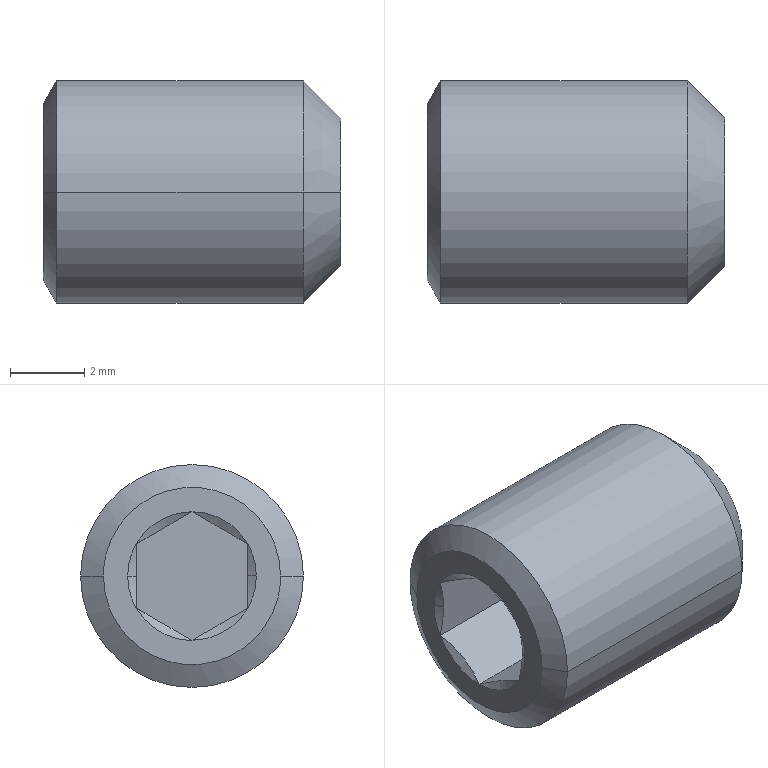Part | STEP file | _Headless pin DIN 913 - M6x8 | 1 solid | 23 faces | box 8 x 6 x 6 mm | volume 188.543 mm3 | cone 12 | plane 9 | cylinder 2 | commonest cylinder face diameters 6 x2
STEP:
#1=CARTESIAN_POINT('',(0.,-1.5,0.866));
#2=VERTEX_POINT('',#1);
#3=CARTESIAN_POINT('',(0.,0.,1.732));
#4=VERTEX_POINT('',#3);
#5=CARTESIAN_POINT('',(0.,-1.5,0.866));
#6=CARTESIAN_POINT('',(0.1211,-1.137,1.075));
#7=CARTESIAN_POINT('',(0.1533,-0.8845,1.221));
#8=CARTESIAN_POINT('',(0.1534,-0.6169,1.377));
#9=CARTESIAN_POINT('',(0.1211,-0.3629,1.522));
#10=CARTESIAN_POINT('',(0.,0.,1.732));
#11=B_SPLINE_CURVE_WITH_KNOTS('',5,(#5,#6,#7,#8,#9,#10),.UNSPECIFIED.,.F.,.U.,(6,6),(0.,104.781),.UNSPECIFIED.);
#12=EDGE_CURVE('',#2,#4,#11,.T.);
#13=ORIENTED_EDGE('',*,*,#12,.F.);
#14=CARTESIAN_POINT('',(0.,0.,0.));
#15=DIRECTION('',(-1.,0.,0.));
#16=AXIS2_PLACEMENT_3D('',#14,#15,$);
#17=CIRCLE('',#16,1.732);
#18=EDGE_CURVE('',#2,#4,#17,.T.);
#19=ORIENTED_EDGE('',*,*,#18,.T.);
#20=EDGE_LOOP('',(#13,#19));
#21=FACE_OUTER_BOUND('',#20,.T.);
#22=CARTESIAN_POINT('',(0.,0.,0.));
#23=DIRECTION('',(-1.,0.,0.));
#24=DIRECTION('',(0.,-1.,0.));
#25=AXIS2_PLACEMENT_3D('',#22,#23,#24);
#26=CONICAL_SURFACE('',#25,1.732,1.047);
#27=ADVANCED_FACE('',(#21),#26,.F.);
#28=ORIENTED_EDGE('',*,*,#12,.T.);
#29=CARTESIAN_POINT('',(3.5,-0.000000001,1.732));
#30=VERTEX_POINT('',#29);
#31=CARTESIAN_POINT('',(1.75,0.,1.732));
#32=DIRECTION('',(-1.,0.,0.));
#33=VECTOR('',#32,1.);
#34=LINE('',#31,#33);
#35=EDGE_CURVE('',#30,#4,#34,.T.);
#36=ORIENTED_EDGE('',*,*,#35,.F.);
#37=CARTESIAN_POINT('',(3.5,-1.5,0.866));
#38=VERTEX_POINT('',#37);
#39=CARTESIAN_POINT('',(3.5,-0.75,1.299));
#40=DIRECTION('',(0.,-0.866,-0.5));
#41=VECTOR('',#40,1.);
#42=LINE('',#39,#41);
#43=EDGE_CURVE('',#30,#38,#42,.T.);
#44=ORIENTED_EDGE('',*,*,#43,.T.);
#45=CARTESIAN_POINT('',(1.75,-1.5,0.866));
#46=DIRECTION('',(-1.,0.,0.));
#47=VECTOR('',#46,1.);
#48=LINE('',#45,#47);
#49=EDGE_CURVE('',#38,#2,#48,.T.);
#50=ORIENTED_EDGE('',*,*,#49,.T.);
#51=EDGE_LOOP('',(#28,#36,#44,#50));
#52=FACE_OUTER_BOUND('',#51,.T.);
#53=CARTESIAN_POINT('',(3.5,0.,1.732));
#54=DIRECTION('',(0.,0.5,-0.866));
#55=DIRECTION('',(0.,0.866,0.5));
#56=AXIS2_PLACEMENT_3D('',#53,#54,#55);
#57=PLANE('',#56);
#58=ADVANCED_FACE('',(#52),#57,.T.);
#59=CARTESIAN_POINT('',(0.,2.386,0.));
#60=VERTEX_POINT('',#59);
#61=CARTESIAN_POINT('',(0.,-2.386,0.));
#62=VERTEX_POINT('',#61);
#63=CARTESIAN_POINT('',(0.,2.387,0.));
#64=CARTESIAN_POINT('',(0.,2.387,-0.227));
#65=CARTESIAN_POINT('',(0.,2.36,-0.4541));
#66=CARTESIAN_POINT('',(0.,2.305,-0.6768));
#67=CARTESIAN_POINT('',(0.,2.146,-1.105));
#68=CARTESIAN_POINT('',(0.,1.89,-1.484));
#69=CARTESIAN_POINT('',(0.,1.74,-1.657));
#70=CARTESIAN_POINT('',(0.,1.401,-1.965));
#71=CARTESIAN_POINT('',(0.,1.,-2.185));
#72=CARTESIAN_POINT('',(0.,0.7874,-2.27));
#73=CARTESIAN_POINT('',(0.,0.3458,-2.389));
#74=CARTESIAN_POINT('',(0.,-0.1114,-2.4));
#75=CARTESIAN_POINT('',(0.,-0.3396,-2.379));
#76=CARTESIAN_POINT('',(0.,-0.7865,-2.282));
#77=CARTESIAN_POINT('',(0.,-1.198,-2.083));
#78=CARTESIAN_POINT('',(0.,-1.391,-1.959));
#79=CARTESIAN_POINT('',(0.,-1.744,-1.668));
#80=CARTESIAN_POINT('',(0.,-2.019,-1.303));
#81=CARTESIAN_POINT('',(0.,-2.134,-1.105));
#82=CARTESIAN_POINT('',(0.,-2.279,-0.7675));
#83=CARTESIAN_POINT('',(0.,-2.357,-0.4107));
#84=CARTESIAN_POINT('',(0.,-2.377,-0.2745));
#85=CARTESIAN_POINT('',(0.,-2.386,-0.1372));
#86=CARTESIAN_POINT('',(0.,-2.386,0.));
#87=B_SPLINE_CURVE_WITH_KNOTS('',5,(#63,#64,#65,#66,#67,#68,#69,#70,#71,#72,#73,#74,#75,#76,#77,#78,#79,#80,#81,#82,#83,#84,#85,#86),.UNSPECIFIED.,.F.,.U.,(6,3,3,3,3,3,3,6),(0.,1.605,3.211,4.816,6.422,8.027,9.633,10.603),.UNSPECIFIED.);
#88=EDGE_CURVE('',#60,#62,#87,.T.);
#89=ORIENTED_EDGE('',*,*,#88,.T.);
#90=CARTESIAN_POINT('',(0.,-2.386,0.));
#91=CARTESIAN_POINT('',(0.,-2.386,0.227));
#92=CARTESIAN_POINT('',(0.,-2.36,0.4541));
#93=CARTESIAN_POINT('',(0.,-2.305,0.6768));
#94=CARTESIAN_POINT('',(0.,-2.146,1.105));
#95=CARTESIAN_POINT('',(0.,-1.89,1.484));
#96=CARTESIAN_POINT('',(0.,-1.74,1.657));
#97=CARTESIAN_POINT('',(0.,-1.401,1.965));
#98=CARTESIAN_POINT('',(0.,-1.,2.185));
#99=CARTESIAN_POINT('',(0.,-0.7874,2.27));
#100=CARTESIAN_POINT('',(0.,-0.3458,2.389));
#101=CARTESIAN_POINT('',(0.,0.1114,2.4));
#102=CARTESIAN_POINT('',(0.,0.3396,2.379));
#103=CARTESIAN_POINT('',(0.,0.7865,2.282));
#104=CARTESIAN_POINT('',(0.,1.198,2.083));
#105=CARTESIAN_POINT('',(0.,1.391,1.959));
#106=CARTESIAN_POINT('',(0.,1.744,1.668));
#107=CARTESIAN_POINT('',(0.,2.019,1.303));
#108=CARTESIAN_POINT('',(0.,2.134,1.105));
#109=CARTESIAN_POINT('',(0.,2.279,0.7675));
#110=CARTESIAN_POINT('',(0.,2.357,0.4107));
#111=CARTESIAN_POINT('',(0.,2.377,0.2745));
#112=CARTESIAN_POINT('',(0.,2.387,0.1372));
#113=CARTESIAN_POINT('',(0.,2.387,0.));
#114=B_SPLINE_CURVE_WITH_KNOTS('',5,(#90,#91,#92,#93,#94,#95,#96,#97,#98,#99,#100,#101,#102,#103,#104,#105,#106,#107,#108,#109,#110,#111,#112,#113),.UNSPECIFIED.,.F.,.U.,(6,3,3,3,3,3,3,6),(0.,1.605,3.211,4.816,6.422,8.027,9.633,10.603),.UNSPECIFIED.);
#115=EDGE_CURVE('',#62,#60,#114,.T.);
#116=ORIENTED_EDGE('',*,*,#115,.T.);
#117=EDGE_LOOP('',(#89,#116));
#118=FACE_OUTER_BOUND('',#117,.T.);
#119=CARTESIAN_POINT('',(0.,-1.732,0.));
#120=VERTEX_POINT('',#119);
#121=CARTESIAN_POINT('',(0.,-1.732,0.));
#122=CARTESIAN_POINT('',(0.,-1.732,0.01204));
#123=CARTESIAN_POINT('',(0.,-1.732,0.02409));
#124=CARTESIAN_POINT('',(0.,-1.732,0.03613));
#125=CARTESIAN_POINT('',(0.,-1.727,0.2175));
#126=CARTESIAN_POINT('',(0.,-1.699,0.3979));
#127=CARTESIAN_POINT('',(0.,-1.651,0.5624));
#128=CARTESIAN_POINT('',(0.,-1.585,0.7194));
#129=CARTESIAN_POINT('',(0.,-1.5,0.866));
#130=B_SPLINE_CURVE_WITH_KNOTS('',5,(#121,#122,#123,#124,#125,#126,#127,#128,#129),.UNSPECIFIED.,.F.,.U.,(6,3,6),(1.283,1.368,2.565),.UNSPECIFIED.);
#131=EDGE_CURVE('',#120,#2,#130,.T.);
#132=ORIENTED_EDGE('',*,*,#131,.F.);
#133=CARTESIAN_POINT('',(0.,-1.5,-0.866));
#134=VERTEX_POINT('',#133);
#135=CARTESIAN_POINT('',(0.,-1.5,-0.866));
#136=CARTESIAN_POINT('',(0.,-1.591,-0.7089));
#137=CARTESIAN_POINT('',(0.,-1.661,-0.54));
#138=CARTESIAN_POINT('',(0.,-1.708,-0.3628));
#139=CARTESIAN_POINT('',(0.,-1.732,-0.1814));
#140=CARTESIAN_POINT('',(0.,-1.732,0.));
#141=B_SPLINE_CURVE_WITH_KNOTS('',5,(#135,#136,#137,#138,#139,#140),.UNSPECIFIED.,.F.,.U.,(6,6),(0.,1.283),.UNSPECIFIED.);
#142=EDGE_CURVE('',#134,#120,#141,.T.);
#143=ORIENTED_EDGE('',*,*,#142,.F.);
#144=CARTESIAN_POINT('',(0.,0.,-1.732));
#145=VERTEX_POINT('',#144);
#146=CARTESIAN_POINT('',(0.,-0.000000001,-1.732));
#147=CARTESIAN_POINT('',(0.,-0.1934,-1.732));
#148=CARTESIAN_POINT('',(0.,-0.3868,-1.705));
#149=CARTESIAN_POINT('',(0.,-0.5752,-1.651));
#150=CARTESIAN_POINT('',(0.,-0.9097,-1.502));
#151=CARTESIAN_POINT('',(0.,-1.194,-1.272));
#152=CARTESIAN_POINT('',(0.,-1.313,-1.149));
#153=CARTESIAN_POINT('',(0.,-1.415,-1.013));
#154=CARTESIAN_POINT('',(0.,-1.5,-0.866));
#155=B_SPLINE_CURVE_WITH_KNOTS('',5,(#146,#147,#148,#149,#150,#151,#152,#153,#154),.UNSPECIFIED.,.F.,.U.,(6,3,6),(0.,1.368,2.565),.UNSPECIFIED.);
#156=EDGE_CURVE('',#145,#134,#155,.T.);
#157=ORIENTED_EDGE('',*,*,#156,.F.);
#158=CARTESIAN_POINT('',(0.,1.5,-0.866));
#159=VERTEX_POINT('',#158);
#160=CARTESIAN_POINT('',(0.,1.5,-0.866));
#161=CARTESIAN_POINT('',(0.,1.403,-1.034));
#162=CARTESIAN_POINT('',(0.,1.283,-1.188));
#163=CARTESIAN_POINT('',(0.,1.142,-1.324));
#164=CARTESIAN_POINT('',(0.,0.8457,-1.539));
#165=CARTESIAN_POINT('',(0.,0.5046,-1.67));
#166=CARTESIAN_POINT('',(0.,0.3387,-1.711));
#167=CARTESIAN_POINT('',(0.,0.1693,-1.732));
#168=CARTESIAN_POINT('',(0.,-0.000000001,-1.732));
#169=B_SPLINE_CURVE_WITH_KNOTS('',5,(#160,#161,#162,#163,#164,#165,#166,#167,#168),.UNSPECIFIED.,.F.,.U.,(6,3,6),(0.,1.368,2.565),.UNSPECIFIED.);
#170=EDGE_CURVE('',#159,#145,#169,.T.);
#171=ORIENTED_EDGE('',*,*,#170,.F.);
#172=CARTESIAN_POINT('',(0.,1.732,0.));
#173=VERTEX_POINT('',#172);
#174=CARTESIAN_POINT('',(0.,1.732,0.));
#175=CARTESIAN_POINT('',(0.,1.732,-0.01204));
#176=CARTESIAN_POINT('',(0.,1.732,-0.02409));
#177=CARTESIAN_POINT('',(0.,1.732,-0.03613));
#178=CARTESIAN_POINT('',(0.,1.727,-0.2175));
#179=CARTESIAN_POINT('',(0.,1.699,-0.3979));
#180=CARTESIAN_POINT('',(0.,1.651,-0.5624));
#181=CARTESIAN_POINT('',(0.,1.585,-0.7194));
#182=CARTESIAN_POINT('',(0.,1.5,-0.866));
#183=B_SPLINE_CURVE_WITH_KNOTS('',5,(#174,#175,#176,#177,#178,#179,#180,#181,#182),.UNSPECIFIED.,.F.,.U.,(6,3,6),(1.283,1.368,2.565),.UNSPECIFIED.);
#184=EDGE_CURVE('',#173,#159,#183,.T.);
#185=ORIENTED_EDGE('',*,*,#184,.F.);
#186=CARTESIAN_POINT('',(0.,1.5,0.866));
#187=VERTEX_POINT('',#186);
#188=CARTESIAN_POINT('',(0.,1.5,0.866));
#189=CARTESIAN_POINT('',(0.,1.591,0.7089));
#190=CARTESIAN_POINT('',(0.,1.661,0.54));
#191=CARTESIAN_POINT('',(0.,1.708,0.3628));
#192=CARTESIAN_POINT('',(0.,1.732,0.1814));
#193=CARTESIAN_POINT('',(0.,1.732,0.));
#194=B_SPLINE_CURVE_WITH_KNOTS('',5,(#188,#189,#190,#191,#192,#193),.UNSPECIFIED.,.F.,.U.,(6,6),(0.,1.283),.UNSPECIFIED.);
#195=EDGE_CURVE('',#187,#173,#194,.T.);
#196=ORIENTED_EDGE('',*,*,#195,.F.);
#197=CARTESIAN_POINT('',(0.,-0.000000001,1.732));
#198=CARTESIAN_POINT('',(0.,0.1934,1.732));
#199=CARTESIAN_POINT('',(0.,0.3868,1.705));
#200=CARTESIAN_POINT('',(0.,0.5752,1.651));
#201=CARTESIAN_POINT('',(0.,0.9097,1.502));
#202=CARTESIAN_POINT('',(0.,1.194,1.272));
#203=CARTESIAN_POINT('',(0.,1.313,1.149));
#204=CARTESIAN_POINT('',(0.,1.415,1.013));
#205=CARTESIAN_POINT('',(0.,1.5,0.866));
#206=B_SPLINE_CURVE_WITH_KNOTS('',5,(#197,#198,#199,#200,#201,#202,#203,#204,#205),.UNSPECIFIED.,.F.,.U.,(6,3,6),(0.,1.368,2.565),.UNSPECIFIED.);
#207=EDGE_CURVE('',#4,#187,#206,.T.);
#208=ORIENTED_EDGE('',*,*,#207,.F.);
#209=ORIENTED_EDGE('',*,*,#18,.F.);
#210=EDGE_LOOP('',(#132,#143,#157,#171,#185,#196,#208,#209));
#211=FACE_BOUND('',#210,.T.);
#212=CARTESIAN_POINT('',(0.,-2.386,0.));
#213=DIRECTION('',(1.,0.,0.));
#214=DIRECTION('',(0.,1.,0.));
#215=AXIS2_PLACEMENT_3D('',#212,#213,#214);
#216=PLANE('',#215);
#217=ADVANCED_FACE('',(#118,#211),#216,.F.);
#218=CARTESIAN_POINT('',(0.,-0.000000001,1.732));
#219=CARTESIAN_POINT('',(0.05807,0.1735,1.632));
#220=CARTESIAN_POINT('',(0.1037,0.3502,1.53));
#221=CARTESIAN_POINT('',(0.1362,0.5392,1.421));
#222=CARTESIAN_POINT('',(0.1461,0.8424,1.246));
#223=CARTESIAN_POINT('',(0.0996,1.143,1.072));
#224=CARTESIAN_POINT('',(0.07278,1.264,1.002));
#225=CARTESIAN_POINT('',(0.03928,1.383,0.9336));
#226=CARTESIAN_POINT('',(0.,1.5,0.866));
#227=B_SPLINE_CURVE_WITH_KNOTS('',5,(#218,#219,#220,#221,#222,#223,#224,#225,#226),.UNSPECIFIED.,.F.,.U.,(6,3,6),(0.,1.478,2.475),.UNSPECIFIED.);
#228=EDGE_CURVE('',#4,#187,#227,.T.);
#229=ORIENTED_EDGE('',*,*,#228,.T.);
#230=CARTESIAN_POINT('',(3.5,1.5,0.866));
#231=VERTEX_POINT('',#230);
#232=CARTESIAN_POINT('',(1.75,1.5,0.866));
#233=DIRECTION('',(-1.,0.,0.));
#234=VECTOR('',#233,1.);
#235=LINE('',#232,#234);
#236=EDGE_CURVE('',#231,#187,#235,.T.);
#237=ORIENTED_EDGE('',*,*,#236,.F.);
#238=CARTESIAN_POINT('',(3.5,0.75,1.299));
#239=DIRECTION('',(0.,-0.866,0.5));
#240=VECTOR('',#239,1.);
#241=LINE('',#238,#240);
#242=EDGE_CURVE('',#231,#30,#241,.T.);
#243=ORIENTED_EDGE('',*,*,#242,.T.);
#244=ORIENTED_EDGE('',*,*,#35,.T.);
#245=EDGE_LOOP('',(#229,#237,#243,#244));
#246=FACE_OUTER_BOUND('',#245,.T.);
#247=CARTESIAN_POINT('',(3.5,1.5,0.866));
#248=DIRECTION('',(0.,-0.5,-0.866));
#249=DIRECTION('',(0.,0.866,-0.5));
#250=AXIS2_PLACEMENT_3D('',#247,#248,#249);
#251=PLANE('',#250);
#252=ADVANCED_FACE('',(#246),#251,.T.);
#253=ORIENTED_EDGE('',*,*,#242,.F.);
#254=CARTESIAN_POINT('',(3.5,1.5,-0.866));
#255=VERTEX_POINT('',#254);
#256=CARTESIAN_POINT('',(3.5,1.5,0.));
#257=DIRECTION('',(0.,0.,1.));
#258=VECTOR('',#257,1.);
#259=LINE('',#256,#258);
#260=EDGE_CURVE('',#255,#231,#259,.T.);
#261=ORIENTED_EDGE('',*,*,#260,.F.);
#262=CARTESIAN_POINT('',(3.5,0.000000001,-1.732));
#263=VERTEX_POINT('',#262);
#264=CARTESIAN_POINT('',(3.5,0.75,-1.299));
#265=DIRECTION('',(0.,0.866,0.5));
#266=VECTOR('',#265,1.);
#267=LINE('',#264,#266);
#268=EDGE_CURVE('',#263,#255,#267,.T.);
#269=ORIENTED_EDGE('',*,*,#268,.F.);
#270=CARTESIAN_POINT('',(3.5,-1.5,-0.866));
#271=VERTEX_POINT('',#270);
#272=CARTESIAN_POINT('',(3.5,-0.75,-1.299));
#273=DIRECTION('',(0.,0.866,-0.5));
#274=VECTOR('',#273,1.);
#275=LINE('',#272,#274);
#276=EDGE_CURVE('',#271,#263,#275,.T.);
#277=ORIENTED_EDGE('',*,*,#276,.F.);
#278=CARTESIAN_POINT('',(3.5,-1.5,0.));
#279=DIRECTION('',(0.,0.,-1.));
#280=VECTOR('',#279,1.);
#281=LINE('',#278,#280);
#282=EDGE_CURVE('',#38,#271,#281,.T.);
#283=ORIENTED_EDGE('',*,*,#282,.F.);
#284=ORIENTED_EDGE('',*,*,#43,.F.);
#285=EDGE_LOOP('',(#253,#261,#269,#277,#283,#284));
#286=FACE_OUTER_BOUND('',#285,.T.);
#287=CARTESIAN_POINT('',(3.5,0.,0.));
#288=DIRECTION('',(1.,0.,0.));
#289=DIRECTION('',(0.,0.,-1.));
#290=AXIS2_PLACEMENT_3D('',#287,#288,#289);
#291=PLANE('',#290);
#292=ADVANCED_FACE('',(#286),#291,.F.);
#293=CARTESIAN_POINT('',(0.134,-1.5,0.000000006));
#294=VERTEX_POINT('',#293);
#295=CARTESIAN_POINT('',(0.,-1.5,-0.866));
#296=CARTESIAN_POINT('',(0.03911,-1.5,-0.7307));
#297=CARTESIAN_POINT('',(0.07296,-1.5,-0.5931));
#298=CARTESIAN_POINT('',(0.1,-1.5,-0.455));
#299=CARTESIAN_POINT('',(0.1233,-1.5,-0.2807));
#300=CARTESIAN_POINT('',(0.1322,-1.5,-0.1053));
#301=CARTESIAN_POINT('',(0.1334,-1.5,-0.07031));
#302=CARTESIAN_POINT('',(0.134,-1.5,-0.0352));
#303=CARTESIAN_POINT('',(0.134,-1.5,-0.00000002));
#304=B_SPLINE_CURVE_WITH_KNOTS('',5,(#295,#296,#297,#298,#299,#300,#301,#302,#303),.UNSPECIFIED.,.F.,.U.,(6,3,6),(0.,0.997,1.245),.UNSPECIFIED.);
#305=EDGE_CURVE('',#134,#294,#304,.T.);
#306=ORIENTED_EDGE('',*,*,#305,.T.);
#307=CARTESIAN_POINT('',(0.134,-1.5,-0.00000002));
#308=CARTESIAN_POINT('',(0.1339,-1.5,0.1056));
#309=CARTESIAN_POINT('',(0.1284,-1.5,0.2121));
#310=CARTESIAN_POINT('',(0.1175,-1.5,0.3189));
#311=CARTESIAN_POINT('',(0.09166,-1.5,0.4924));
#312=CARTESIAN_POINT('',(0.05418,-1.5,0.6632));
#313=CARTESIAN_POINT('',(0.03749,-1.5,0.7312));
#314=CARTESIAN_POINT('',(0.01936,-1.5,0.7988));
#315=CARTESIAN_POINT('',(0.,-1.5,0.866));
#316=B_SPLINE_CURVE_WITH_KNOTS('',5,(#307,#308,#309,#310,#311,#312,#313,#314,#315),.UNSPECIFIED.,.F.,.U.,(6,3,6),(1.245,1.987,2.484),.UNSPECIFIED.);
#317=EDGE_CURVE('',#294,#2,#316,.T.);
#318=ORIENTED_EDGE('',*,*,#317,.T.);
#319=ORIENTED_EDGE('',*,*,#49,.F.);
#320=ORIENTED_EDGE('',*,*,#282,.T.);
#321=CARTESIAN_POINT('',(1.75,-1.5,-0.866));
#322=DIRECTION('',(-1.,0.,0.));
#323=VECTOR('',#322,1.);
#324=LINE('',#321,#323);
#325=EDGE_CURVE('',#271,#134,#324,.T.);
#326=ORIENTED_EDGE('',*,*,#325,.T.);
#327=EDGE_LOOP('',(#306,#318,#319,#320,#326));
#328=FACE_OUTER_BOUND('',#327,.T.);
#329=CARTESIAN_POINT('',(3.5,-1.5,0.866));
#330=DIRECTION('',(0.,1.,0.));
#331=DIRECTION('',(0.,0.,1.));
#332=AXIS2_PLACEMENT_3D('',#329,#330,#331);
#333=PLANE('',#332);
#334=ADVANCED_FACE('',(#328),#333,.T.);
#335=CARTESIAN_POINT('',(0.3542,-3.,0.));
#336=VERTEX_POINT('',#335);
#337=CARTESIAN_POINT('',(249999.488,-433014.202,0.));
#338=DIRECTION('',(0.5,-0.866,0.));
#339=VECTOR('',#338,1.);
#340=LINE('',#337,#339);
#341=EDGE_CURVE('',#62,#336,#340,.T.);
#342=ORIENTED_EDGE('',*,*,#341,.F.);
#343=ORIENTED_EDGE('',*,*,#88,.F.);
#344=CARTESIAN_POINT('',(0.3542,3.,0.));
#345=VERTEX_POINT('',#344);
#346=CARTESIAN_POINT('',(249999.488,433014.202,0.));
#347=DIRECTION('',(0.5,0.866,0.));
#348=VECTOR('',#347,1.);
#349=LINE('',#346,#348);
#350=EDGE_CURVE('',#345,#60,#349,.F.);
#351=ORIENTED_EDGE('',*,*,#350,.F.);
#352=CARTESIAN_POINT('',(0.3542,0.,0.));
#353=DIRECTION('',(1.,0.,0.));
#354=AXIS2_PLACEMENT_3D('',#352,#353,$);
#355=CIRCLE('',#354,3.);
#356=EDGE_CURVE('',#345,#336,#355,.F.);
#357=ORIENTED_EDGE('',*,*,#356,.T.);
#358=EDGE_LOOP('',(#342,#343,#351,#357));
#359=FACE_OUTER_BOUND('',#358,.T.);
#360=CARTESIAN_POINT('',(0.3542,0.,0.));
#361=DIRECTION('',(1.,0.,0.));
#362=DIRECTION('',(0.,-1.,0.));
#363=AXIS2_PLACEMENT_3D('',#360,#361,#362);
#364=CONICAL_SURFACE('',#363,3.,1.047);
#365=ADVANCED_FACE('',(#359),#364,.T.);
#366=ORIENTED_EDGE('',*,*,#350,.T.);
#367=ORIENTED_EDGE('',*,*,#115,.F.);
#368=ORIENTED_EDGE('',*,*,#341,.T.);
#369=CARTESIAN_POINT('',(0.3542,0.,0.));
#370=DIRECTION('',(1.,0.,0.));
#371=AXIS2_PLACEMENT_3D('',#369,#370,$);
#372=CIRCLE('',#371,3.);
#373=EDGE_CURVE('',#336,#345,#372,.F.);
#374=ORIENTED_EDGE('',*,*,#373,.T.);
#375=EDGE_LOOP('',(#366,#367,#368,#374));
#376=FACE_OUTER_BOUND('',#375,.T.);
#377=CARTESIAN_POINT('',(0.3542,0.,0.));
#378=DIRECTION('',(1.,0.,0.));
#379=DIRECTION('',(0.,1.,0.));
#380=AXIS2_PLACEMENT_3D('',#377,#378,#379);
#381=CONICAL_SURFACE('',#380,3.,1.047);
#382=ADVANCED_FACE('',(#376),#381,.T.);
#383=ORIENTED_EDGE('',*,*,#131,.T.);
#384=ORIENTED_EDGE('',*,*,#317,.F.);
#385=CARTESIAN_POINT('',(-249999.5,-433013.568,0.));
#386=DIRECTION('',(-0.5,-0.866,0.));
#387=VECTOR('',#386,1.);
#388=LINE('',#385,#387);
#389=EDGE_CURVE('',#120,#294,#388,.F.);
#390=ORIENTED_EDGE('',*,*,#389,.F.);
#391=EDGE_LOOP('',(#383,#384,#390));
#392=FACE_OUTER_BOUND('',#391,.T.);
#393=CARTESIAN_POINT('',(0.,0.,0.));
#394=DIRECTION('',(-1.,0.,0.));
#395=DIRECTION('',(0.,-1.,0.));
#396=AXIS2_PLACEMENT_3D('',#393,#394,#395);
#397=CONICAL_SURFACE('',#396,1.732,1.047);
#398=ADVANCED_FACE('',(#392),#397,.F.);
#399=ORIENTED_EDGE('',*,*,#305,.F.);
#400=ORIENTED_EDGE('',*,*,#142,.T.);
#401=ORIENTED_EDGE('',*,*,#389,.T.);
#402=EDGE_LOOP('',(#399,#400,#401));
#403=FACE_OUTER_BOUND('',#402,.T.);
#404=CARTESIAN_POINT('',(0.,0.,0.));
#405=DIRECTION('',(-1.,0.,0.));
#406=DIRECTION('',(0.,1.,0.));
#407=AXIS2_PLACEMENT_3D('',#404,#405,#406);
#408=CONICAL_SURFACE('',#407,1.732,1.047);
#409=ADVANCED_FACE('',(#403),#408,.F.);
#410=CARTESIAN_POINT('',(0.,0.,-1.732));
#411=CARTESIAN_POINT('',(0.1211,-0.3629,-1.522));
#412=CARTESIAN_POINT('',(0.1533,-0.6156,-1.377));
#413=CARTESIAN_POINT('',(0.1534,-0.8837,-1.223));
#414=CARTESIAN_POINT('',(0.1211,-1.137,-1.075));
#415=CARTESIAN_POINT('',(0.,-1.5,-0.866));
#416=B_SPLINE_CURVE_WITH_KNOTS('',5,(#410,#411,#412,#413,#414,#415),.UNSPECIFIED.,.F.,.U.,(6,6),(0.,104.781),.UNSPECIFIED.);
#417=EDGE_CURVE('',#145,#134,#416,.T.);
#418=ORIENTED_EDGE('',*,*,#417,.F.);
#419=ORIENTED_EDGE('',*,*,#156,.T.);
#420=EDGE_LOOP('',(#418,#419));
#421=FACE_OUTER_BOUND('',#420,.T.);
#422=CARTESIAN_POINT('',(0.,0.,0.));
#423=DIRECTION('',(-1.,0.,0.));
#424=DIRECTION('',(0.,1.,0.));
#425=AXIS2_PLACEMENT_3D('',#422,#423,#424);
#426=CONICAL_SURFACE('',#425,1.732,1.047);
#427=ADVANCED_FACE('',(#421),#426,.F.);
#428=CARTESIAN_POINT('',(0.,1.5,-0.866));
#429=CARTESIAN_POINT('',(0.1211,1.137,-1.075));
#430=CARTESIAN_POINT('',(0.1533,0.8845,-1.221));
#431=CARTESIAN_POINT('',(0.1534,0.6169,-1.377));
#432=CARTESIAN_POINT('',(0.1211,0.3629,-1.522));
#433=CARTESIAN_POINT('',(0.,0.,-1.732));
#434=B_SPLINE_CURVE_WITH_KNOTS('',5,(#428,#429,#430,#431,#432,#433),.UNSPECIFIED.,.F.,.U.,(6,6),(0.,104.781),.UNSPECIFIED.);
#435=EDGE_CURVE('',#159,#145,#434,.T.);
#436=ORIENTED_EDGE('',*,*,#435,.F.);
#437=ORIENTED_EDGE('',*,*,#170,.T.);
#438=EDGE_LOOP('',(#436,#437));
#439=FACE_OUTER_BOUND('',#438,.T.);
#440=CARTESIAN_POINT('',(0.,0.,0.));
#441=DIRECTION('',(-1.,0.,0.));
#442=DIRECTION('',(0.,1.,0.));
#443=AXIS2_PLACEMENT_3D('',#440,#441,#442);
#444=CONICAL_SURFACE('',#443,1.732,1.047);
#445=ADVANCED_FACE('',(#439),#444,.F.);
#446=ORIENTED_EDGE('',*,*,#184,.T.);
#447=CARTESIAN_POINT('',(0.134,1.5,0.));
#448=VERTEX_POINT('',#447);
#449=CARTESIAN_POINT('',(0.,1.5,-0.866));
#450=CARTESIAN_POINT('',(0.07581,1.5,-0.6035));
#451=CARTESIAN_POINT('',(0.1136,1.5,-0.3939));
#452=CARTESIAN_POINT('',(0.134,1.5,-0.1969));
#453=CARTESIAN_POINT('',(0.134,1.5,0.));
#454=B_SPLINE_CURVE_WITH_KNOTS('',4,(#449,#450,#451,#452,#453),.UNSPECIFIED.,.F.,.U.,(5,5),(0.,52.521),.UNSPECIFIED.);
#455=EDGE_CURVE('',#448,#159,#454,.F.);
#456=ORIENTED_EDGE('',*,*,#455,.F.);
#457=CARTESIAN_POINT('',(-249999.5,433013.568,0.));
#458=DIRECTION('',(-0.5,0.866,0.));
#459=VECTOR('',#458,1.);
#460=LINE('',#457,#459);
#461=EDGE_CURVE('',#448,#173,#460,.T.);
#462=ORIENTED_EDGE('',*,*,#461,.T.);
#463=EDGE_LOOP('',(#446,#456,#462));
#464=FACE_OUTER_BOUND('',#463,.T.);
#465=CARTESIAN_POINT('',(0.,0.,0.));
#466=DIRECTION('',(-1.,0.,0.));
#467=DIRECTION('',(0.,1.,0.));
#468=AXIS2_PLACEMENT_3D('',#465,#466,#467);
#469=CONICAL_SURFACE('',#468,1.732,1.047);
#470=ADVANCED_FACE('',(#464),#469,.F.);
#471=CARTESIAN_POINT('',(0.134,1.5,0.));
#472=CARTESIAN_POINT('',(0.1339,1.5,0.1962));
#473=CARTESIAN_POINT('',(0.1137,1.5,0.3943));
#474=CARTESIAN_POINT('',(0.07547,1.5,0.6045));
#475=CARTESIAN_POINT('',(0.,1.5,0.866));
#476=B_SPLINE_CURVE_WITH_KNOTS('',4,(#471,#472,#473,#474,#475),.UNSPECIFIED.,.F.,.U.,(5,5),(0.,52.333),.UNSPECIFIED.);
#477=EDGE_CURVE('',#187,#448,#476,.F.);
#478=ORIENTED_EDGE('',*,*,#477,.F.);
#479=ORIENTED_EDGE('',*,*,#195,.T.);
#480=ORIENTED_EDGE('',*,*,#461,.F.);
#481=EDGE_LOOP('',(#478,#479,#480));
#482=FACE_OUTER_BOUND('',#481,.T.);
#483=CARTESIAN_POINT('',(0.,0.,0.));
#484=DIRECTION('',(-1.,0.,0.));
#485=DIRECTION('',(0.,-1.,0.));
#486=AXIS2_PLACEMENT_3D('',#483,#484,#485);
#487=CONICAL_SURFACE('',#486,1.732,1.047);
#488=ADVANCED_FACE('',(#482),#487,.F.);
#489=ORIENTED_EDGE('',*,*,#228,.F.);
#490=ORIENTED_EDGE('',*,*,#207,.T.);
#491=EDGE_LOOP('',(#489,#490));
#492=FACE_OUTER_BOUND('',#491,.T.);
#493=CARTESIAN_POINT('',(0.,0.,0.));
#494=DIRECTION('',(-1.,0.,0.));
#495=DIRECTION('',(0.,-1.,0.));
#496=AXIS2_PLACEMENT_3D('',#493,#494,#495);
#497=CONICAL_SURFACE('',#496,1.732,1.047);
#498=ADVANCED_FACE('',(#492),#497,.F.);
#499=ORIENTED_EDGE('',*,*,#477,.T.);
#500=ORIENTED_EDGE('',*,*,#455,.T.);
#501=CARTESIAN_POINT('',(1.75,1.5,-0.866));
#502=DIRECTION('',(-1.,0.,0.));
#503=VECTOR('',#502,1.);
#504=LINE('',#501,#503);
#505=EDGE_CURVE('',#255,#159,#504,.T.);
#506=ORIENTED_EDGE('',*,*,#505,.F.);
#507=ORIENTED_EDGE('',*,*,#260,.T.);
#508=ORIENTED_EDGE('',*,*,#236,.T.);
#509=EDGE_LOOP('',(#499,#500,#506,#507,#508));
#510=FACE_OUTER_BOUND('',#509,.T.);
#511=CARTESIAN_POINT('',(3.5,1.5,-0.866));
#512=DIRECTION('',(0.,-1.,0.));
#513=DIRECTION('',(0.,0.,-1.));
#514=AXIS2_PLACEMENT_3D('',#511,#512,#513);
#515=PLANE('',#514);
#516=ADVANCED_FACE('',(#510),#515,.T.);
#517=ORIENTED_EDGE('',*,*,#435,.T.);
#518=CARTESIAN_POINT('',(1.75,0.,-1.732));
#519=DIRECTION('',(-1.,0.,0.));
#520=VECTOR('',#519,1.);
#521=LINE('',#518,#520);
#522=EDGE_CURVE('',#263,#145,#521,.T.);
#523=ORIENTED_EDGE('',*,*,#522,.F.);
#524=ORIENTED_EDGE('',*,*,#268,.T.);
#525=ORIENTED_EDGE('',*,*,#505,.T.);
#526=EDGE_LOOP('',(#517,#523,#524,#525));
#527=FACE_OUTER_BOUND('',#526,.T.);
#528=CARTESIAN_POINT('',(3.5,0.,-1.732));
#529=DIRECTION('',(0.,-0.5,0.866));
#530=DIRECTION('',(0.,-0.866,-0.5));
#531=AXIS2_PLACEMENT_3D('',#528,#529,#530);
#532=PLANE('',#531);
#533=ADVANCED_FACE('',(#527),#532,.T.);
#534=ORIENTED_EDGE('',*,*,#417,.T.);
#535=ORIENTED_EDGE('',*,*,#325,.F.);
#536=ORIENTED_EDGE('',*,*,#276,.T.);
#537=ORIENTED_EDGE('',*,*,#522,.T.);
#538=EDGE_LOOP('',(#534,#535,#536,#537));
#539=FACE_OUTER_BOUND('',#538,.T.);
#540=CARTESIAN_POINT('',(3.5,-1.5,-0.866));
#541=DIRECTION('',(0.,0.5,0.866));
#542=DIRECTION('',(0.,-0.866,0.5));
#543=AXIS2_PLACEMENT_3D('',#540,#541,#542);
#544=PLANE('',#543);
#545=ADVANCED_FACE('',(#539),#544,.T.);
#546=CARTESIAN_POINT('',(7.,3.,0.));
#547=VERTEX_POINT('',#546);
#548=CARTESIAN_POINT('',(1.,3.,0.));
#549=DIRECTION('',(1.,0.,0.));
#550=VECTOR('',#549,1.);
#551=LINE('',#548,#550);
#552=EDGE_CURVE('',#345,#547,#551,.T.);
#553=ORIENTED_EDGE('',*,*,#552,.T.);
#554=CARTESIAN_POINT('',(7.,-3.,0.));
#555=VERTEX_POINT('',#554);
#556=CARTESIAN_POINT('',(7.,0.,0.));
#557=DIRECTION('',(1.,0.,0.));
#558=AXIS2_PLACEMENT_3D('',#556,#557,$);
#559=CIRCLE('',#558,3.);
#560=EDGE_CURVE('',#547,#555,#559,.F.);
#561=ORIENTED_EDGE('',*,*,#560,.T.);
#562=CARTESIAN_POINT('',(1.,-3.,0.));
#563=DIRECTION('',(1.,0.,0.));
#564=VECTOR('',#563,1.);
#565=LINE('',#562,#564);
#566=EDGE_CURVE('',#555,#336,#565,.F.);
#567=ORIENTED_EDGE('',*,*,#566,.T.);
#568=ORIENTED_EDGE('',*,*,#356,.F.);
#569=EDGE_LOOP('',(#553,#561,#567,#568));
#570=FACE_OUTER_BOUND('',#569,.T.);
#571=CARTESIAN_POINT('',(1.,0.,0.));
#572=DIRECTION('',(1.,0.,0.));
#573=DIRECTION('',(0.,-1.,0.));
#574=AXIS2_PLACEMENT_3D('',#571,#572,#573);
#575=CYLINDRICAL_SURFACE('',#574,3.);
#576=ADVANCED_FACE('',(#570),#575,.T.);
#577=ORIENTED_EDGE('',*,*,#566,.F.);
#578=CARTESIAN_POINT('',(7.,0.,0.));
#579=DIRECTION('',(1.,0.,0.));
#580=AXIS2_PLACEMENT_3D('',#578,#579,$);
#581=CIRCLE('',#580,3.);
#582=EDGE_CURVE('',#555,#547,#581,.F.);
#583=ORIENTED_EDGE('',*,*,#582,.T.);
#584=ORIENTED_EDGE('',*,*,#552,.F.);
#585=ORIENTED_EDGE('',*,*,#373,.F.);
#586=EDGE_LOOP('',(#577,#583,#584,#585));
#587=FACE_OUTER_BOUND('',#586,.T.);
#588=CARTESIAN_POINT('',(1.,0.,0.));
#589=DIRECTION('',(1.,0.,0.));
#590=DIRECTION('',(0.,1.,0.));
#591=AXIS2_PLACEMENT_3D('',#588,#589,#590);
#592=CYLINDRICAL_SURFACE('',#591,3.);
#593=ADVANCED_FACE('',(#587),#592,.T.);
#594=CARTESIAN_POINT('',(8.,2.,0.));
#595=VERTEX_POINT('',#594);
#596=CARTESIAN_POINT('',(-353544.391,353554.391,0.));
#597=DIRECTION('',(-0.7071,0.7071,0.));
#598=VECTOR('',#597,1.);
#599=LINE('',#596,#598);
#600=EDGE_CURVE('',#595,#547,#599,.T.);
#601=ORIENTED_EDGE('',*,*,#600,.F.);
#602=CARTESIAN_POINT('',(8.,-2.,0.));
#603=VERTEX_POINT('',#602);
#604=CARTESIAN_POINT('',(8.,0.,0.));
#605=DIRECTION('',(-1.,0.,0.));
#606=AXIS2_PLACEMENT_3D('',#604,#605,$);
#607=CIRCLE('',#606,2.);
#608=EDGE_CURVE('',#595,#603,#607,.T.);
#609=ORIENTED_EDGE('',*,*,#608,.T.);
#610=CARTESIAN_POINT('',(-353544.391,-353554.391,0.));
#611=DIRECTION('',(-0.7071,-0.7071,0.));
#612=VECTOR('',#611,1.);
#613=LINE('',#610,#612);
#614=EDGE_CURVE('',#555,#603,#613,.F.);
#615=ORIENTED_EDGE('',*,*,#614,.F.);
#616=ORIENTED_EDGE('',*,*,#560,.F.);
#617=EDGE_LOOP('',(#601,#609,#615,#616));
#618=FACE_OUTER_BOUND('',#617,.T.);
#619=CARTESIAN_POINT('',(8.,0.,0.));
#620=DIRECTION('',(-1.,0.,0.));
#621=DIRECTION('',(0.,1.,0.));
#622=AXIS2_PLACEMENT_3D('',#619,#620,#621);
#623=CONICAL_SURFACE('',#622,2.,0.7854);
#624=ADVANCED_FACE('',(#618),#623,.T.);
#625=ORIENTED_EDGE('',*,*,#614,.T.);
#626=CARTESIAN_POINT('',(8.,0.,0.));
#627=DIRECTION('',(-1.,0.,0.));
#628=AXIS2_PLACEMENT_3D('',#626,#627,$);
#629=CIRCLE('',#628,2.);
#630=EDGE_CURVE('',#603,#595,#629,.T.);
#631=ORIENTED_EDGE('',*,*,#630,.T.);
#632=ORIENTED_EDGE('',*,*,#600,.T.);
#633=ORIENTED_EDGE('',*,*,#582,.F.);
#634=EDGE_LOOP('',(#625,#631,#632,#633));
#635=FACE_OUTER_BOUND('',#634,.T.);
#636=CARTESIAN_POINT('',(8.,0.,0.));
#637=DIRECTION('',(-1.,0.,0.));
#638=DIRECTION('',(0.,-1.,0.));
#639=AXIS2_PLACEMENT_3D('',#636,#637,#638);
#640=CONICAL_SURFACE('',#639,2.,0.7854);
#641=ADVANCED_FACE('',(#635),#640,.T.);
#642=ORIENTED_EDGE('',*,*,#630,.F.);
#643=ORIENTED_EDGE('',*,*,#608,.F.);
#644=EDGE_LOOP('',(#642,#643));
#645=FACE_OUTER_BOUND('',#644,.T.);
#646=CARTESIAN_POINT('',(8.,0.,0.));
#647=DIRECTION('',(-1.,0.,0.));
#648=DIRECTION('',(0.,-1.,0.));
#649=AXIS2_PLACEMENT_3D('',#646,#647,#648);
#650=PLANE('',#649);
#651=ADVANCED_FACE('',(#645),#650,.F.);
#652=CLOSED_SHELL('',(#27,#58,#217,#252,#292,#334,#365,#382,#398,#409,#427,#445,#470,#488,#498,#516,#533,#545,#576,#593,#624,#641,#651));
#653=MANIFOLD_SOLID_BREP('',#652);
#654=(LENGTH_UNIT()NAMED_UNIT(*)SI_UNIT(.MILLI.,.METRE.));
#655=UNCERTAINTY_MEASURE_WITH_UNIT(LENGTH_MEASURE(0.005),#654,'','');
#656=(NAMED_UNIT(*)PLANE_ANGLE_UNIT()SI_UNIT($,.RADIAN.));
#657=(NAMED_UNIT(*)SI_UNIT($,.STERADIAN.)SOLID_ANGLE_UNIT());
#658=(GEOMETRIC_REPRESENTATION_CONTEXT(3)GLOBAL_UNCERTAINTY_ASSIGNED_CONTEXT((#655))GLOBAL_UNIT_ASSIGNED_CONTEXT((#654,#656,#657))REPRESENTATION_CONTEXT('',''));
#659=ADVANCED_BREP_SHAPE_REPRESENTATION('',(#653),#658);